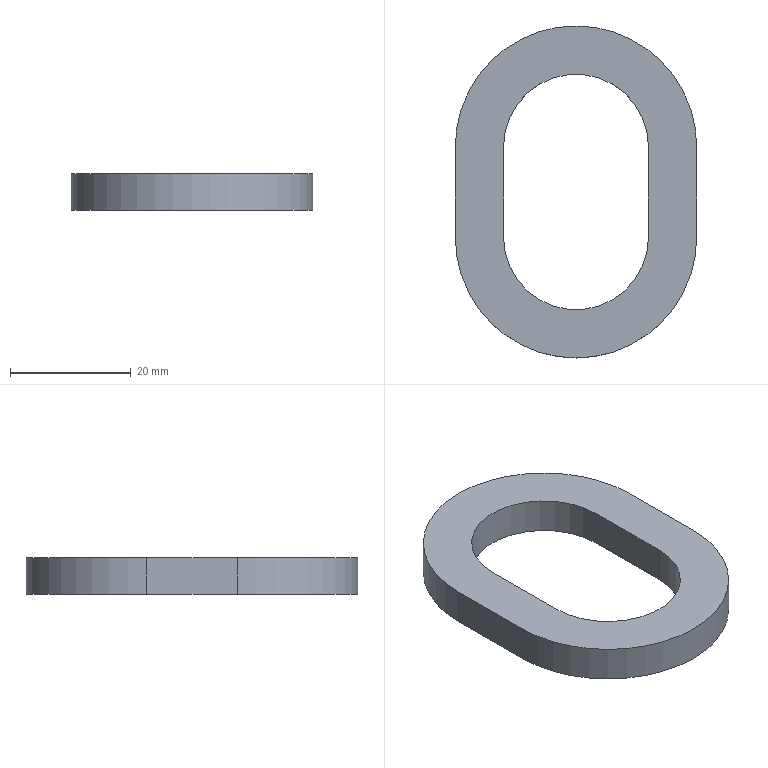Part | SolidWorks | features FlatPattern 1, SMBaseFlange 1, SheetMetal 1 | 1 solid | 10 faces | box 40 x 55 x 6 mm | volume 6265 mm3 | plane 6 | cylinder 4 | commonest cylinder face diameters 24 x2 40 x2
STEP:
#1=CARTESIAN_POINT('',(50.973,41.57,0.));
#2=VERTEX_POINT('',#1);
#3=CARTESIAN_POINT('',(10.973,41.57,0.));
#4=VERTEX_POINT('',#3);
#5=CARTESIAN_POINT('',(30.973,41.57,0.));
#6=DIRECTION('',(0.,0.,1.));
#7=DIRECTION('',(1.,0.,0.));
#8=AXIS2_PLACEMENT_3D('',#5,#6,#7);
#9=CIRCLE('',#8,20.);
#10=EDGE_CURVE('',#2,#4,#9,.T.);
#11=ORIENTED_EDGE('',*,*,#10,.F.);
#12=CARTESIAN_POINT('',(50.973,41.57,-6.));
#13=VERTEX_POINT('',#12);
#14=CARTESIAN_POINT('',(50.973,41.57,-6.));
#15=DIRECTION('',(0.,0.,1.));
#16=VECTOR('',#15,1000.);
#17=LINE('',#14,#16);
#18=EDGE_CURVE('',#13,#2,#17,.T.);
#19=ORIENTED_EDGE('',*,*,#18,.F.);
#20=CARTESIAN_POINT('',(10.973,41.57,-6.));
#21=VERTEX_POINT('',#20);
#22=CARTESIAN_POINT('',(30.973,41.57,-6.));
#23=DIRECTION('',(0.,0.,1.));
#24=DIRECTION('',(1.,0.,0.));
#25=AXIS2_PLACEMENT_3D('',#22,#23,#24);
#26=CIRCLE('',#25,20.);
#27=EDGE_CURVE('',#13,#21,#26,.T.);
#28=ORIENTED_EDGE('',*,*,#27,.T.);
#29=CARTESIAN_POINT('',(10.973,41.57,-6.));
#30=DIRECTION('',(0.,0.,1.));
#31=VECTOR('',#30,1000.);
#32=LINE('',#29,#31);
#33=EDGE_CURVE('',#21,#4,#32,.T.);
#34=ORIENTED_EDGE('',*,*,#33,.T.);
#35=EDGE_LOOP('',(#11,#19,#28,#34));
#36=FACE_OUTER_BOUND('',#35,.T.);
#37=CARTESIAN_POINT('',(30.973,41.57,-6.));
#38=DIRECTION('',(0.,0.,1.));
#39=DIRECTION('',(1.,0.,0.));
#40=AXIS2_PLACEMENT_3D('',#37,#38,#39);
#41=CYLINDRICAL_SURFACE('',#40,20.);
#42=ADVANCED_FACE('',(#36),#41,.T.);
#43=CARTESIAN_POINT('',(50.973,26.57,0.));
#44=VERTEX_POINT('',#43);
#45=CARTESIAN_POINT('',(50.973,26.57,0.));
#46=DIRECTION('',(0.,1.,0.));
#47=VECTOR('',#46,1000.);
#48=LINE('',#45,#47);
#49=EDGE_CURVE('',#44,#2,#48,.T.);
#50=ORIENTED_EDGE('',*,*,#49,.F.);
#51=CARTESIAN_POINT('',(50.973,26.57,-6.));
#52=VERTEX_POINT('',#51);
#53=CARTESIAN_POINT('',(50.973,26.57,-6.));
#54=DIRECTION('',(0.,0.,1.));
#55=VECTOR('',#54,1000.);
#56=LINE('',#53,#55);
#57=EDGE_CURVE('',#52,#44,#56,.T.);
#58=ORIENTED_EDGE('',*,*,#57,.F.);
#59=CARTESIAN_POINT('',(50.973,26.57,-6.));
#60=DIRECTION('',(0.,1.,0.));
#61=VECTOR('',#60,1000.);
#62=LINE('',#59,#61);
#63=EDGE_CURVE('',#52,#13,#62,.T.);
#64=ORIENTED_EDGE('',*,*,#63,.T.);
#65=ORIENTED_EDGE('',*,*,#18,.T.);
#66=EDGE_LOOP('',(#50,#58,#64,#65));
#67=FACE_OUTER_BOUND('',#66,.T.);
#68=CARTESIAN_POINT('',(50.973,26.57,-6.));
#69=DIRECTION('',(1.,0.,0.));
#70=DIRECTION('',(0.,0.,-1.));
#71=AXIS2_PLACEMENT_3D('',#68,#69,#70);
#72=PLANE('',#71);
#73=ADVANCED_FACE('',(#67),#72,.T.);
#74=CARTESIAN_POINT('',(10.973,26.57,0.));
#75=VERTEX_POINT('',#74);
#76=CARTESIAN_POINT('',(30.973,26.57,0.));
#77=DIRECTION('',(0.,0.,1.));
#78=DIRECTION('',(1.,0.,0.));
#79=AXIS2_PLACEMENT_3D('',#76,#77,#78);
#80=CIRCLE('',#79,20.);
#81=EDGE_CURVE('',#75,#44,#80,.T.);
#82=ORIENTED_EDGE('',*,*,#81,.F.);
#83=CARTESIAN_POINT('',(10.973,26.57,-6.));
#84=VERTEX_POINT('',#83);
#85=CARTESIAN_POINT('',(10.973,26.57,-6.));
#86=DIRECTION('',(0.,0.,1.));
#87=VECTOR('',#86,1000.);
#88=LINE('',#85,#87);
#89=EDGE_CURVE('',#84,#75,#88,.T.);
#90=ORIENTED_EDGE('',*,*,#89,.F.);
#91=CARTESIAN_POINT('',(30.973,26.57,-6.));
#92=DIRECTION('',(0.,0.,1.));
#93=DIRECTION('',(1.,0.,0.));
#94=AXIS2_PLACEMENT_3D('',#91,#92,#93);
#95=CIRCLE('',#94,20.);
#96=EDGE_CURVE('',#84,#52,#95,.T.);
#97=ORIENTED_EDGE('',*,*,#96,.T.);
#98=ORIENTED_EDGE('',*,*,#57,.T.);
#99=EDGE_LOOP('',(#82,#90,#97,#98));
#100=FACE_OUTER_BOUND('',#99,.T.);
#101=CARTESIAN_POINT('',(30.973,26.57,-6.));
#102=DIRECTION('',(0.,0.,1.));
#103=DIRECTION('',(1.,0.,0.));
#104=AXIS2_PLACEMENT_3D('',#101,#102,#103);
#105=CYLINDRICAL_SURFACE('',#104,20.);
#106=ADVANCED_FACE('',(#100),#105,.T.);
#107=CARTESIAN_POINT('',(10.973,41.57,0.));
#108=DIRECTION('',(0.,-1.,0.));
#109=VECTOR('',#108,1000.);
#110=LINE('',#107,#109);
#111=EDGE_CURVE('',#4,#75,#110,.T.);
#112=ORIENTED_EDGE('',*,*,#111,.F.);
#113=ORIENTED_EDGE('',*,*,#33,.F.);
#114=CARTESIAN_POINT('',(10.973,41.57,-6.));
#115=DIRECTION('',(0.,-1.,0.));
#116=VECTOR('',#115,1000.);
#117=LINE('',#114,#116);
#118=EDGE_CURVE('',#21,#84,#117,.T.);
#119=ORIENTED_EDGE('',*,*,#118,.T.);
#120=ORIENTED_EDGE('',*,*,#89,.T.);
#121=EDGE_LOOP('',(#112,#113,#119,#120));
#122=FACE_OUTER_BOUND('',#121,.T.);
#123=CARTESIAN_POINT('',(10.973,41.57,-6.));
#124=DIRECTION('',(-1.,0.,0.));
#125=DIRECTION('',(0.,-1.,0.));
#126=AXIS2_PLACEMENT_3D('',#123,#124,#125);
#127=PLANE('',#126);
#128=ADVANCED_FACE('',(#122),#127,.T.);
#129=CARTESIAN_POINT('',(42.973,26.57,-6.));
#130=VERTEX_POINT('',#129);
#131=CARTESIAN_POINT('',(42.973,41.57,-6.));
#132=VERTEX_POINT('',#131);
#133=CARTESIAN_POINT('',(42.973,26.57,-6.));
#134=DIRECTION('',(0.,1.,0.));
#135=VECTOR('',#134,1000.);
#136=LINE('',#133,#135);
#137=EDGE_CURVE('',#130,#132,#136,.T.);
#138=ORIENTED_EDGE('',*,*,#137,.T.);
#139=CARTESIAN_POINT('',(18.973,41.57,-6.));
#140=VERTEX_POINT('',#139);
#141=CARTESIAN_POINT('',(30.973,41.57,-6.));
#142=DIRECTION('',(0.,0.,1.));
#143=DIRECTION('',(1.,0.,0.));
#144=AXIS2_PLACEMENT_3D('',#141,#142,#143);
#145=CIRCLE('',#144,12.);
#146=EDGE_CURVE('',#132,#140,#145,.T.);
#147=ORIENTED_EDGE('',*,*,#146,.T.);
#148=CARTESIAN_POINT('',(18.973,26.57,-6.));
#149=VERTEX_POINT('',#148);
#150=CARTESIAN_POINT('',(18.973,41.57,-6.));
#151=DIRECTION('',(0.,-1.,0.));
#152=VECTOR('',#151,1000.);
#153=LINE('',#150,#152);
#154=EDGE_CURVE('',#140,#149,#153,.T.);
#155=ORIENTED_EDGE('',*,*,#154,.T.);
#156=CARTESIAN_POINT('',(30.973,26.57,-6.));
#157=DIRECTION('',(0.,0.,1.));
#158=DIRECTION('',(1.,0.,0.));
#159=AXIS2_PLACEMENT_3D('',#156,#157,#158);
#160=CIRCLE('',#159,12.);
#161=EDGE_CURVE('',#149,#130,#160,.T.);
#162=ORIENTED_EDGE('',*,*,#161,.T.);
#163=EDGE_LOOP('',(#138,#147,#155,#162));
#164=FACE_BOUND('',#163,.T.);
#165=ORIENTED_EDGE('',*,*,#27,.F.);
#166=ORIENTED_EDGE('',*,*,#63,.F.);
#167=ORIENTED_EDGE('',*,*,#96,.F.);
#168=ORIENTED_EDGE('',*,*,#118,.F.);
#169=EDGE_LOOP('',(#165,#166,#167,#168));
#170=FACE_OUTER_BOUND('',#169,.T.);
#171=CARTESIAN_POINT('',(30.973,41.57,-6.));
#172=DIRECTION('',(0.,0.,1.));
#173=DIRECTION('',(1.,0.,0.));
#174=AXIS2_PLACEMENT_3D('',#171,#172,#173);
#175=PLANE('',#174);
#176=ADVANCED_FACE('',(#164,#170),#175,.F.);
#177=CARTESIAN_POINT('',(42.973,41.57,0.));
#178=VERTEX_POINT('',#177);
#179=CARTESIAN_POINT('',(18.973,41.57,0.));
#180=VERTEX_POINT('',#179);
#181=CARTESIAN_POINT('',(30.973,41.57,0.));
#182=DIRECTION('',(0.,0.,1.));
#183=DIRECTION('',(1.,0.,0.));
#184=AXIS2_PLACEMENT_3D('',#181,#182,#183);
#185=CIRCLE('',#184,12.);
#186=EDGE_CURVE('',#178,#180,#185,.T.);
#187=ORIENTED_EDGE('',*,*,#186,.F.);
#188=CARTESIAN_POINT('',(42.973,26.57,0.));
#189=VERTEX_POINT('',#188);
#190=CARTESIAN_POINT('',(42.973,26.57,0.));
#191=DIRECTION('',(0.,1.,0.));
#192=VECTOR('',#191,1000.);
#193=LINE('',#190,#192);
#194=EDGE_CURVE('',#189,#178,#193,.T.);
#195=ORIENTED_EDGE('',*,*,#194,.F.);
#196=CARTESIAN_POINT('',(18.973,26.57,0.));
#197=VERTEX_POINT('',#196);
#198=CARTESIAN_POINT('',(30.973,26.57,0.));
#199=DIRECTION('',(0.,0.,1.));
#200=DIRECTION('',(1.,0.,0.));
#201=AXIS2_PLACEMENT_3D('',#198,#199,#200);
#202=CIRCLE('',#201,12.);
#203=EDGE_CURVE('',#197,#189,#202,.T.);
#204=ORIENTED_EDGE('',*,*,#203,.F.);
#205=CARTESIAN_POINT('',(18.973,41.57,0.));
#206=DIRECTION('',(0.,-1.,0.));
#207=VECTOR('',#206,1000.);
#208=LINE('',#205,#207);
#209=EDGE_CURVE('',#180,#197,#208,.T.);
#210=ORIENTED_EDGE('',*,*,#209,.F.);
#211=EDGE_LOOP('',(#187,#195,#204,#210));
#212=FACE_BOUND('',#211,.T.);
#213=ORIENTED_EDGE('',*,*,#10,.T.);
#214=ORIENTED_EDGE('',*,*,#111,.T.);
#215=ORIENTED_EDGE('',*,*,#81,.T.);
#216=ORIENTED_EDGE('',*,*,#49,.T.);
#217=EDGE_LOOP('',(#213,#214,#215,#216));
#218=FACE_OUTER_BOUND('',#217,.T.);
#219=CARTESIAN_POINT('',(30.973,41.57,0.));
#220=DIRECTION('',(0.,0.,1.));
#221=DIRECTION('',(1.,0.,0.));
#222=AXIS2_PLACEMENT_3D('',#219,#220,#221);
#223=PLANE('',#222);
#224=ADVANCED_FACE('',(#212,#218),#223,.T.);
#225=ORIENTED_EDGE('',*,*,#186,.T.);
#226=CARTESIAN_POINT('',(18.973,41.57,-6.));
#227=DIRECTION('',(0.,0.,1.));
#228=VECTOR('',#227,1000.);
#229=LINE('',#226,#228);
#230=EDGE_CURVE('',#140,#180,#229,.T.);
#231=ORIENTED_EDGE('',*,*,#230,.F.);
#232=ORIENTED_EDGE('',*,*,#146,.F.);
#233=CARTESIAN_POINT('',(42.973,41.57,-6.));
#234=DIRECTION('',(0.,0.,1.));
#235=VECTOR('',#234,1000.);
#236=LINE('',#233,#235);
#237=EDGE_CURVE('',#132,#178,#236,.T.);
#238=ORIENTED_EDGE('',*,*,#237,.T.);
#239=EDGE_LOOP('',(#225,#231,#232,#238));
#240=FACE_OUTER_BOUND('',#239,.T.);
#241=CARTESIAN_POINT('',(30.973,41.57,-6.));
#242=DIRECTION('',(0.,0.,1.));
#243=DIRECTION('',(1.,0.,0.));
#244=AXIS2_PLACEMENT_3D('',#241,#242,#243);
#245=CYLINDRICAL_SURFACE('',#244,12.);
#246=ADVANCED_FACE('',(#240),#245,.F.);
#247=ORIENTED_EDGE('',*,*,#194,.T.);
#248=ORIENTED_EDGE('',*,*,#237,.F.);
#249=ORIENTED_EDGE('',*,*,#137,.F.);
#250=CARTESIAN_POINT('',(42.973,26.57,-6.));
#251=DIRECTION('',(0.,0.,1.));
#252=VECTOR('',#251,1000.);
#253=LINE('',#250,#252);
#254=EDGE_CURVE('',#130,#189,#253,.T.);
#255=ORIENTED_EDGE('',*,*,#254,.T.);
#256=EDGE_LOOP('',(#247,#248,#249,#255));
#257=FACE_OUTER_BOUND('',#256,.T.);
#258=CARTESIAN_POINT('',(42.973,26.57,-6.));
#259=DIRECTION('',(1.,0.,0.));
#260=DIRECTION('',(0.,1.,0.));
#261=AXIS2_PLACEMENT_3D('',#258,#259,#260);
#262=PLANE('',#261);
#263=ADVANCED_FACE('',(#257),#262,.F.);
#264=ORIENTED_EDGE('',*,*,#203,.T.);
#265=ORIENTED_EDGE('',*,*,#254,.F.);
#266=ORIENTED_EDGE('',*,*,#161,.F.);
#267=CARTESIAN_POINT('',(18.973,26.57,-6.));
#268=DIRECTION('',(0.,0.,1.));
#269=VECTOR('',#268,1000.);
#270=LINE('',#267,#269);
#271=EDGE_CURVE('',#149,#197,#270,.T.);
#272=ORIENTED_EDGE('',*,*,#271,.T.);
#273=EDGE_LOOP('',(#264,#265,#266,#272));
#274=FACE_OUTER_BOUND('',#273,.T.);
#275=CARTESIAN_POINT('',(30.973,26.57,-6.));
#276=DIRECTION('',(0.,0.,1.));
#277=DIRECTION('',(1.,0.,0.));
#278=AXIS2_PLACEMENT_3D('',#275,#276,#277);
#279=CYLINDRICAL_SURFACE('',#278,12.);
#280=ADVANCED_FACE('',(#274),#279,.F.);
#281=ORIENTED_EDGE('',*,*,#209,.T.);
#282=ORIENTED_EDGE('',*,*,#271,.F.);
#283=ORIENTED_EDGE('',*,*,#154,.F.);
#284=ORIENTED_EDGE('',*,*,#230,.T.);
#285=EDGE_LOOP('',(#281,#282,#283,#284));
#286=FACE_OUTER_BOUND('',#285,.T.);
#287=CARTESIAN_POINT('',(18.973,41.57,-6.));
#288=DIRECTION('',(-1.,0.,0.));
#289=DIRECTION('',(0.,-1.,0.));
#290=AXIS2_PLACEMENT_3D('',#287,#288,#289);
#291=PLANE('',#290);
#292=ADVANCED_FACE('',(#286),#291,.F.);
#293=CLOSED_SHELL('',(#42,#73,#106,#128,#176,#224,#246,#263,#280,#292));
#294=MANIFOLD_SOLID_BREP('',#293);
#295=CARTESIAN_POINT('',(0.,0.,0.));
#296=DIRECTION('',(0.,0.,1.));
#297=DIRECTION('',(1.,0.,0.));
#298=AXIS2_PLACEMENT_3D('',#295,#296,#297);
#299=(LENGTH_UNIT()NAMED_UNIT(*)SI_UNIT(.MILLI.,.METRE.));
#300=UNCERTAINTY_MEASURE_WITH_UNIT(LENGTH_MEASURE(0.00001),#299,'','');
#301=(NAMED_UNIT(*)PLANE_ANGLE_UNIT()SI_UNIT($,.RADIAN.));
#302=(NAMED_UNIT(*)SI_UNIT($,.STERADIAN.)SOLID_ANGLE_UNIT());
#303=(GEOMETRIC_REPRESENTATION_CONTEXT(3)GLOBAL_UNCERTAINTY_ASSIGNED_CONTEXT((#300))GLOBAL_UNIT_ASSIGNED_CONTEXT((#299,#301,#302))REPRESENTATION_CONTEXT('',''));
#304=ADVANCED_BREP_SHAPE_REPRESENTATION('',(#294,#298),#303);